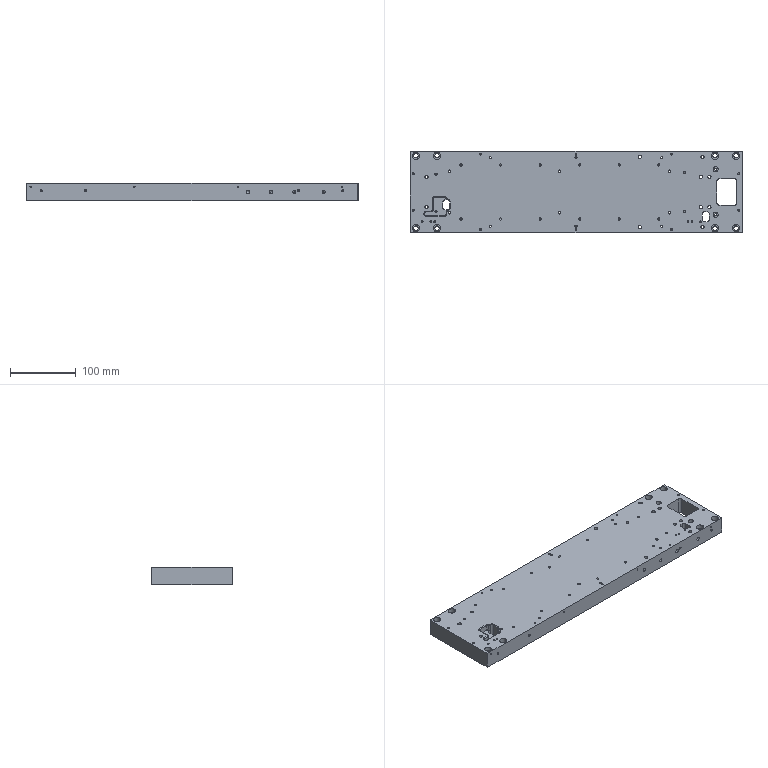Part | STEP file | 1 solid | 398 faces | box 504 x 124 x 26 mm | volume 1554634 mm3 | cylinder 227 | cone 127 | plane 44 | commonest cylinder face diameters 3.3 x72 5 x36 2.5 x24 6 x19 2.05 x16 6.8 x16